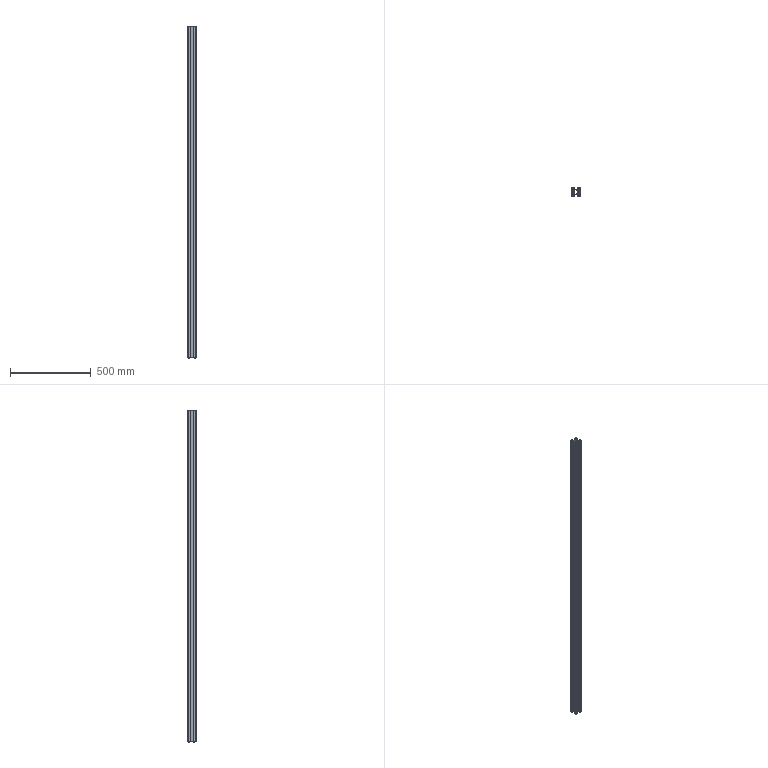Part | STEP file | 46A-00006CC11-2050mm | 1 solid | 142 faces | box 50 x 50 x 2050 mm | volume 1204359 mm3 | cylinder 84 | plane 58 | commonest cylinder face diameters 1 x24 4 x24 1.5 x16 3.7 x8 6.7 x8 2 x4